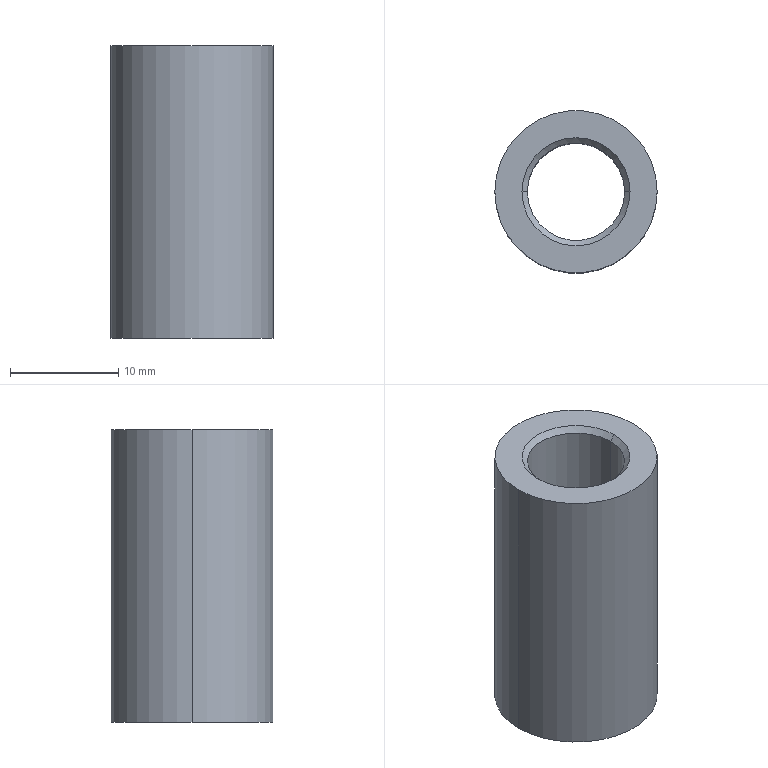Part | STEP file | Ngam kep 8 | 1 solid | 10 faces | box 15 x 15 x 27 mm | volume 3046 mm3 | cone 4 | cylinder 4 | plane 2 | commonest cylinder face diameters 9 x2 15 x2
STEP:
#1=CARTESIAN_POINT('',(0.,0.,0.));
#2=DIRECTION('',(0.,0.,1.));
#3=DIRECTION('',(1.,0.,0.));
#4=AXIS2_PLACEMENT_3D('',#1,#2,#3);
#5=CARTESIAN_POINT('',(4.5,0.,26.5));
#6=VERTEX_POINT('',#5);
#7=CARTESIAN_POINT('',(5.,0.,27.));
#8=VERTEX_POINT('',#7);
#9=CARTESIAN_POINT('',(4.5,0.,26.5));
#10=DIRECTION('',(0.7071,0.,0.7071));
#11=VECTOR('',#10,1.);
#12=LINE('',#9,#11);
#13=CARTESIAN_POINT('',(0.,0.,26.5));
#14=DIRECTION('',(0.,0.,1.));
#15=DIRECTION('',(1.,0.,0.));
#16=AXIS2_PLACEMENT_3D('',#13,#14,#15);
#17=CONICAL_SURFACE('',#16,4.5,0.7854);
#18=CARTESIAN_POINT('',(6.283,0.));
#19=DIRECTION('',(0.,1.));
#20=VECTOR('',#19,1.);
#21=LINE('',#18,#20);
#22=(GEOMETRIC_REPRESENTATION_CONTEXT(2)PARAMETRIC_REPRESENTATION_CONTEXT()REPRESENTATION_CONTEXT('',''));
#23=DEFINITIONAL_REPRESENTATION('',(#21),#22);
#24=PCURVE('',#17,#23);
#25=CARTESIAN_POINT('',(0.,0.,26.5));
#26=DIRECTION('',(0.,0.,1.));
#27=DIRECTION('',(1.,0.,0.));
#28=AXIS2_PLACEMENT_3D('',#25,#26,#27);
#29=CONICAL_SURFACE('',#28,4.5,0.7854);
#30=CARTESIAN_POINT('',(0.,0.));
#31=DIRECTION('',(0.,1.));
#32=VECTOR('',#31,1.);
#33=LINE('',#30,#32);
#34=(GEOMETRIC_REPRESENTATION_CONTEXT(2)PARAMETRIC_REPRESENTATION_CONTEXT()REPRESENTATION_CONTEXT('',''));
#35=DEFINITIONAL_REPRESENTATION('',(#33),#34);
#36=PCURVE('',#29,#35);
#37=SURFACE_CURVE('',#12,(#24,#36),.PCURVE_S1.);
#38=EDGE_CURVE('',#6,#8,#37,.T.);
#39=ORIENTED_EDGE('',*,*,#38,.T.);
#40=CARTESIAN_POINT('',(-5.,0.,27.));
#41=VERTEX_POINT('',#40);
#42=CARTESIAN_POINT('',(0.,0.,27.));
#43=DIRECTION('',(0.,0.,-1.));
#44=DIRECTION('',(1.,0.,0.));
#45=AXIS2_PLACEMENT_3D('',#42,#43,#44);
#46=CIRCLE('',#45,5.);
#47=CARTESIAN_POINT('',(6.283,0.5));
#48=DIRECTION('',(-1.,0.));
#49=VECTOR('',#48,1.);
#50=LINE('',#47,#49);
#51=(GEOMETRIC_REPRESENTATION_CONTEXT(2)PARAMETRIC_REPRESENTATION_CONTEXT()REPRESENTATION_CONTEXT('',''));
#52=DEFINITIONAL_REPRESENTATION('',(#50),#51);
#53=PCURVE('',#17,#52);
#54=CARTESIAN_POINT('',(0.,0.,27.));
#55=DIRECTION('',(0.,0.,1.));
#56=DIRECTION('',(1.,0.,0.));
#57=AXIS2_PLACEMENT_3D('',#54,#55,#56);
#58=PLANE('',#57);
#59=CARTESIAN_POINT('',(5.,0.));
#60=CARTESIAN_POINT('',(5.,-8.66));
#61=CARTESIAN_POINT('',(-2.5,-4.33));
#62=CARTESIAN_POINT('',(-10.,0.));
#63=CARTESIAN_POINT('',(-2.5,4.33));
#64=CARTESIAN_POINT('',(5.,8.66));
#65=CARTESIAN_POINT('',(5.,0.));
#66=(BOUNDED_CURVE()B_SPLINE_CURVE(2,(#59,#60,#61,#62,#63,#64,#65),.UNSPECIFIED.,.T.,.F.)B_SPLINE_CURVE_WITH_KNOTS((1,2,2,2,2,1),(-2.094,0.,2.094,4.189,6.283,8.378),.UNSPECIFIED.)CURVE()GEOMETRIC_REPRESENTATION_ITEM()RATIONAL_B_SPLINE_CURVE((1.,0.5,1.,0.5,1.,0.5,1.))REPRESENTATION_ITEM(''));
#67=(GEOMETRIC_REPRESENTATION_CONTEXT(2)PARAMETRIC_REPRESENTATION_CONTEXT()REPRESENTATION_CONTEXT('',''));
#68=DEFINITIONAL_REPRESENTATION('',(#66),#67);
#69=PCURVE('',#58,#68);
#70=SURFACE_CURVE('',#46,(#53,#69),.PCURVE_S1.);
#71=EDGE_CURVE('',#8,#41,#70,.T.);
#72=ORIENTED_EDGE('',*,*,#71,.T.);
#73=CARTESIAN_POINT('',(-4.5,0.,26.5));
#74=VERTEX_POINT('',#73);
#75=CARTESIAN_POINT('',(-4.5,0.,26.5));
#76=DIRECTION('',(-0.7071,0.,0.7071));
#77=VECTOR('',#76,1.);
#78=LINE('',#75,#77);
#79=CARTESIAN_POINT('',(3.142,0.));
#80=DIRECTION('',(0.,1.));
#81=VECTOR('',#80,1.);
#82=LINE('',#79,#81);
#83=(GEOMETRIC_REPRESENTATION_CONTEXT(2)PARAMETRIC_REPRESENTATION_CONTEXT()REPRESENTATION_CONTEXT('',''));
#84=DEFINITIONAL_REPRESENTATION('',(#82),#83);
#85=PCURVE('',#17,#84);
#86=CARTESIAN_POINT('',(3.142,0.));
#87=DIRECTION('',(0.,1.));
#88=VECTOR('',#87,1.);
#89=LINE('',#86,#88);
#90=(GEOMETRIC_REPRESENTATION_CONTEXT(2)PARAMETRIC_REPRESENTATION_CONTEXT()REPRESENTATION_CONTEXT('',''));
#91=DEFINITIONAL_REPRESENTATION('',(#89),#90);
#92=PCURVE('',#29,#91);
#93=SURFACE_CURVE('',#78,(#85,#92),.PCURVE_S1.);
#94=EDGE_CURVE('',#74,#41,#93,.T.);
#95=ORIENTED_EDGE('',*,*,#94,.F.);
#96=CARTESIAN_POINT('',(0.,0.,26.5));
#97=DIRECTION('',(0.,0.,1.));
#98=DIRECTION('',(1.,0.,0.));
#99=AXIS2_PLACEMENT_3D('',#96,#97,#98);
#100=CIRCLE('',#99,4.5);
#101=CARTESIAN_POINT('',(0.,0.));
#102=DIRECTION('',(1.,0.));
#103=VECTOR('',#102,1.);
#104=LINE('',#101,#103);
#105=(GEOMETRIC_REPRESENTATION_CONTEXT(2)PARAMETRIC_REPRESENTATION_CONTEXT()REPRESENTATION_CONTEXT('',''));
#106=DEFINITIONAL_REPRESENTATION('',(#104),#105);
#107=PCURVE('',#17,#106);
#108=CARTESIAN_POINT('',(0.,0.,27.));
#109=DIRECTION('',(0.,0.,-1.));
#110=DIRECTION('',(-1.,0.,0.));
#111=AXIS2_PLACEMENT_3D('',#108,#109,#110);
#112=CYLINDRICAL_SURFACE('',#111,4.5);
#113=CARTESIAN_POINT('',(9.425,0.5));
#114=DIRECTION('',(-1.,0.));
#115=VECTOR('',#114,1.);
#116=LINE('',#113,#115);
#117=(GEOMETRIC_REPRESENTATION_CONTEXT(2)PARAMETRIC_REPRESENTATION_CONTEXT()REPRESENTATION_CONTEXT('',''));
#118=DEFINITIONAL_REPRESENTATION('',(#116),#117);
#119=PCURVE('',#112,#118);
#120=SURFACE_CURVE('',#100,(#107,#119),.PCURVE_S1.);
#121=EDGE_CURVE('',#74,#6,#120,.T.);
#122=ORIENTED_EDGE('',*,*,#121,.T.);
#123=EDGE_LOOP('',(#39,#72,#95,#122));
#124=FACE_BOUND('',#123,.F.);
#125=ADVANCED_FACE('',(#124),#17,.F.);
#126=CARTESIAN_POINT('',(-4.5,0.,0.5));
#127=VERTEX_POINT('',#126);
#128=CARTESIAN_POINT('',(-5.,0.,0.));
#129=VERTEX_POINT('',#128);
#130=CARTESIAN_POINT('',(-5.,0.,0.));
#131=DIRECTION('',(-0.7071,0.,-0.7071));
#132=VECTOR('',#131,1.);
#133=LINE('',#130,#132);
#134=CARTESIAN_POINT('',(0.,0.,0.));
#135=DIRECTION('',(0.,0.,-1.));
#136=DIRECTION('',(-1.,0.,0.));
#137=AXIS2_PLACEMENT_3D('',#134,#135,#136);
#138=CONICAL_SURFACE('',#137,5.,0.7854);
#139=CARTESIAN_POINT('',(6.283,0.));
#140=DIRECTION('',(0.,1.));
#141=VECTOR('',#140,1.);
#142=LINE('',#139,#141);
#143=(GEOMETRIC_REPRESENTATION_CONTEXT(2)PARAMETRIC_REPRESENTATION_CONTEXT()REPRESENTATION_CONTEXT('',''));
#144=DEFINITIONAL_REPRESENTATION('',(#142),#143);
#145=PCURVE('',#138,#144);
#146=CARTESIAN_POINT('',(0.,0.,0.));
#147=DIRECTION('',(0.,0.,-1.));
#148=DIRECTION('',(-1.,0.,0.));
#149=AXIS2_PLACEMENT_3D('',#146,#147,#148);
#150=CONICAL_SURFACE('',#149,5.,0.7854);
#151=CARTESIAN_POINT('',(0.,0.));
#152=DIRECTION('',(0.,1.));
#153=VECTOR('',#152,1.);
#154=LINE('',#151,#153);
#155=(GEOMETRIC_REPRESENTATION_CONTEXT(2)PARAMETRIC_REPRESENTATION_CONTEXT()REPRESENTATION_CONTEXT('',''));
#156=DEFINITIONAL_REPRESENTATION('',(#154),#155);
#157=PCURVE('',#150,#156);
#158=SURFACE_CURVE('',#133,(#145,#157),.PCURVE_S1.);
#159=EDGE_CURVE('',#127,#129,#158,.T.);
#160=ORIENTED_EDGE('',*,*,#159,.T.);
#161=CARTESIAN_POINT('',(5.,0.,0.));
#162=VERTEX_POINT('',#161);
#163=CARTESIAN_POINT('',(0.,0.,0.));
#164=DIRECTION('',(0.,0.,1.));
#165=DIRECTION('',(1.,0.,0.));
#166=AXIS2_PLACEMENT_3D('',#163,#164,#165);
#167=CIRCLE('',#166,5.);
#168=CARTESIAN_POINT('',(9.425,0.));
#169=DIRECTION('',(-1.,0.));
#170=VECTOR('',#169,1.);
#171=LINE('',#168,#170);
#172=(GEOMETRIC_REPRESENTATION_CONTEXT(2)PARAMETRIC_REPRESENTATION_CONTEXT()REPRESENTATION_CONTEXT('',''));
#173=DEFINITIONAL_REPRESENTATION('',(#171),#172);
#174=PCURVE('',#138,#173);
#175=CARTESIAN_POINT('',(0.,0.,0.));
#176=DIRECTION('',(0.,0.,1.));
#177=DIRECTION('',(1.,0.,0.));
#178=AXIS2_PLACEMENT_3D('',#175,#176,#177);
#179=PLANE('',#178);
#180=CARTESIAN_POINT('',(0.,0.));
#181=DIRECTION('',(1.,0.));
#182=AXIS2_PLACEMENT_2D('',#180,#181);
#183=CIRCLE('',#182,5.);
#184=(GEOMETRIC_REPRESENTATION_CONTEXT(2)PARAMETRIC_REPRESENTATION_CONTEXT()REPRESENTATION_CONTEXT('',''));
#185=DEFINITIONAL_REPRESENTATION('',(#183),#184);
#186=PCURVE('',#179,#185);
#187=SURFACE_CURVE('',#167,(#174,#186),.PCURVE_S1.);
#188=EDGE_CURVE('',#129,#162,#187,.T.);
#189=ORIENTED_EDGE('',*,*,#188,.T.);
#190=CARTESIAN_POINT('',(4.5,0.,0.5));
#191=VERTEX_POINT('',#190);
#192=CARTESIAN_POINT('',(5.,0.,0.));
#193=DIRECTION('',(0.7071,0.,-0.7071));
#194=VECTOR('',#193,1.);
#195=LINE('',#192,#194);
#196=CARTESIAN_POINT('',(3.142,0.));
#197=DIRECTION('',(0.,1.));
#198=VECTOR('',#197,1.);
#199=LINE('',#196,#198);
#200=(GEOMETRIC_REPRESENTATION_CONTEXT(2)PARAMETRIC_REPRESENTATION_CONTEXT()REPRESENTATION_CONTEXT('',''));
#201=DEFINITIONAL_REPRESENTATION('',(#199),#200);
#202=PCURVE('',#138,#201);
#203=CARTESIAN_POINT('',(3.142,0.));
#204=DIRECTION('',(0.,1.));
#205=VECTOR('',#204,1.);
#206=LINE('',#203,#205);
#207=(GEOMETRIC_REPRESENTATION_CONTEXT(2)PARAMETRIC_REPRESENTATION_CONTEXT()REPRESENTATION_CONTEXT('',''));
#208=DEFINITIONAL_REPRESENTATION('',(#206),#207);
#209=PCURVE('',#150,#208);
#210=SURFACE_CURVE('',#195,(#202,#209),.PCURVE_S1.);
#211=EDGE_CURVE('',#191,#162,#210,.T.);
#212=ORIENTED_EDGE('',*,*,#211,.F.);
#213=CARTESIAN_POINT('',(0.,0.,0.5));
#214=DIRECTION('',(0.,0.,-1.));
#215=DIRECTION('',(1.,0.,0.));
#216=AXIS2_PLACEMENT_3D('',#213,#214,#215);
#217=CIRCLE('',#216,4.5);
#218=CARTESIAN_POINT('',(3.142,-0.5));
#219=DIRECTION('',(1.,0.));
#220=VECTOR('',#219,1.);
#221=LINE('',#218,#220);
#222=(GEOMETRIC_REPRESENTATION_CONTEXT(2)PARAMETRIC_REPRESENTATION_CONTEXT()REPRESENTATION_CONTEXT('',''));
#223=DEFINITIONAL_REPRESENTATION('',(#221),#222);
#224=PCURVE('',#138,#223);
#225=CARTESIAN_POINT('',(3.142,26.5));
#226=DIRECTION('',(1.,0.));
#227=VECTOR('',#226,1.);
#228=LINE('',#225,#227);
#229=(GEOMETRIC_REPRESENTATION_CONTEXT(2)PARAMETRIC_REPRESENTATION_CONTEXT()REPRESENTATION_CONTEXT('',''));
#230=DEFINITIONAL_REPRESENTATION('',(#228),#229);
#231=PCURVE('',#112,#230);
#232=SURFACE_CURVE('',#217,(#224,#231),.PCURVE_S1.);
#233=EDGE_CURVE('',#191,#127,#232,.T.);
#234=ORIENTED_EDGE('',*,*,#233,.T.);
#235=EDGE_LOOP('',(#160,#189,#212,#234));
#236=FACE_BOUND('',#235,.F.);
#237=ADVANCED_FACE('',(#236),#138,.F.);
#238=CARTESIAN_POINT('',(-4.5,0.,27.));
#239=DIRECTION('',(0.,0.,-1.));
#240=VECTOR('',#239,1.);
#241=LINE('',#238,#240);
#242=CARTESIAN_POINT('',(6.283,0.));
#243=DIRECTION('',(0.,1.));
#244=VECTOR('',#243,1.);
#245=LINE('',#242,#244);
#246=(GEOMETRIC_REPRESENTATION_CONTEXT(2)PARAMETRIC_REPRESENTATION_CONTEXT()REPRESENTATION_CONTEXT('',''));
#247=DEFINITIONAL_REPRESENTATION('',(#245),#246);
#248=PCURVE('',#112,#247);
#249=CARTESIAN_POINT('',(0.,0.,27.));
#250=DIRECTION('',(0.,0.,-1.));
#251=DIRECTION('',(-1.,0.,0.));
#252=AXIS2_PLACEMENT_3D('',#249,#250,#251);
#253=CYLINDRICAL_SURFACE('',#252,4.5);
#254=CARTESIAN_POINT('',(0.,0.));
#255=DIRECTION('',(0.,1.));
#256=VECTOR('',#255,1.);
#257=LINE('',#254,#256);
#258=(GEOMETRIC_REPRESENTATION_CONTEXT(2)PARAMETRIC_REPRESENTATION_CONTEXT()REPRESENTATION_CONTEXT('',''));
#259=DEFINITIONAL_REPRESENTATION('',(#257),#258);
#260=PCURVE('',#253,#259);
#261=SURFACE_CURVE('',#241,(#248,#260),.PCURVE_S1.);
#262=EDGE_CURVE('',#74,#127,#261,.T.);
#263=ORIENTED_EDGE('',*,*,#262,.T.);
#264=ORIENTED_EDGE('',*,*,#233,.F.);
#265=CARTESIAN_POINT('',(4.5,0.,27.));
#266=DIRECTION('',(0.,0.,-1.));
#267=VECTOR('',#266,1.);
#268=LINE('',#265,#267);
#269=CARTESIAN_POINT('',(3.142,0.));
#270=DIRECTION('',(0.,1.));
#271=VECTOR('',#270,1.);
#272=LINE('',#269,#271);
#273=(GEOMETRIC_REPRESENTATION_CONTEXT(2)PARAMETRIC_REPRESENTATION_CONTEXT()REPRESENTATION_CONTEXT('',''));
#274=DEFINITIONAL_REPRESENTATION('',(#272),#273);
#275=PCURVE('',#112,#274);
#276=CARTESIAN_POINT('',(3.142,0.));
#277=DIRECTION('',(0.,1.));
#278=VECTOR('',#277,1.);
#279=LINE('',#276,#278);
#280=(GEOMETRIC_REPRESENTATION_CONTEXT(2)PARAMETRIC_REPRESENTATION_CONTEXT()REPRESENTATION_CONTEXT('',''));
#281=DEFINITIONAL_REPRESENTATION('',(#279),#280);
#282=PCURVE('',#253,#281);
#283=SURFACE_CURVE('',#268,(#275,#282),.PCURVE_S1.);
#284=EDGE_CURVE('',#6,#191,#283,.T.);
#285=ORIENTED_EDGE('',*,*,#284,.F.);
#286=ORIENTED_EDGE('',*,*,#121,.F.);
#287=EDGE_LOOP('',(#263,#264,#285,#286));
#288=FACE_BOUND('',#287,.F.);
#289=ADVANCED_FACE('',(#288),#112,.F.);
#290=CARTESIAN_POINT('',(7.5,0.,27.));
#291=VERTEX_POINT('',#290);
#292=CARTESIAN_POINT('',(-7.5,0.,27.));
#293=VERTEX_POINT('',#292);
#294=CARTESIAN_POINT('',(0.,0.,27.));
#295=DIRECTION('',(0.,0.,1.));
#296=DIRECTION('',(1.,0.,0.));
#297=AXIS2_PLACEMENT_3D('',#294,#295,#296);
#298=CIRCLE('',#297,7.5);
#299=CARTESIAN_POINT('',(0.,0.,27.));
#300=DIRECTION('',(0.,0.,-1.));
#301=DIRECTION('',(-1.,0.,0.));
#302=AXIS2_PLACEMENT_3D('',#299,#300,#301);
#303=CYLINDRICAL_SURFACE('',#302,7.5);
#304=CARTESIAN_POINT('',(3.142,0.));
#305=DIRECTION('',(-1.,0.));
#306=VECTOR('',#305,1.);
#307=LINE('',#304,#306);
#308=(GEOMETRIC_REPRESENTATION_CONTEXT(2)PARAMETRIC_REPRESENTATION_CONTEXT()REPRESENTATION_CONTEXT('',''));
#309=DEFINITIONAL_REPRESENTATION('',(#307),#308);
#310=PCURVE('',#303,#309);
#311=CARTESIAN_POINT('',(0.,0.));
#312=DIRECTION('',(1.,0.));
#313=AXIS2_PLACEMENT_2D('',#311,#312);
#314=CIRCLE('',#313,7.5);
#315=(GEOMETRIC_REPRESENTATION_CONTEXT(2)PARAMETRIC_REPRESENTATION_CONTEXT()REPRESENTATION_CONTEXT('',''));
#316=DEFINITIONAL_REPRESENTATION('',(#314),#315);
#317=PCURVE('',#58,#316);
#318=SURFACE_CURVE('',#298,(#310,#317),.PCURVE_S1.);
#319=EDGE_CURVE('',#291,#293,#318,.T.);
#320=ORIENTED_EDGE('',*,*,#319,.F.);
#321=CARTESIAN_POINT('',(7.5,0.,0.));
#322=VERTEX_POINT('',#321);
#323=CARTESIAN_POINT('',(7.5,0.,27.));
#324=DIRECTION('',(0.,0.,-1.));
#325=VECTOR('',#324,1.);
#326=LINE('',#323,#325);
#327=CARTESIAN_POINT('',(3.142,0.));
#328=DIRECTION('',(0.,1.));
#329=VECTOR('',#328,1.);
#330=LINE('',#327,#329);
#331=(GEOMETRIC_REPRESENTATION_CONTEXT(2)PARAMETRIC_REPRESENTATION_CONTEXT()REPRESENTATION_CONTEXT('',''));
#332=DEFINITIONAL_REPRESENTATION('',(#330),#331);
#333=PCURVE('',#303,#332);
#334=CARTESIAN_POINT('',(0.,0.,27.));
#335=DIRECTION('',(0.,0.,-1.));
#336=DIRECTION('',(-1.,0.,0.));
#337=AXIS2_PLACEMENT_3D('',#334,#335,#336);
#338=CYLINDRICAL_SURFACE('',#337,7.5);
#339=CARTESIAN_POINT('',(3.142,0.));
#340=DIRECTION('',(0.,1.));
#341=VECTOR('',#340,1.);
#342=LINE('',#339,#341);
#343=(GEOMETRIC_REPRESENTATION_CONTEXT(2)PARAMETRIC_REPRESENTATION_CONTEXT()REPRESENTATION_CONTEXT('',''));
#344=DEFINITIONAL_REPRESENTATION('',(#342),#343);
#345=PCURVE('',#338,#344);
#346=SURFACE_CURVE('',#326,(#333,#345),.PCURVE_S1.);
#347=EDGE_CURVE('',#291,#322,#346,.T.);
#348=ORIENTED_EDGE('',*,*,#347,.T.);
#349=CARTESIAN_POINT('',(-7.5,0.,0.));
#350=VERTEX_POINT('',#349);
#351=CARTESIAN_POINT('',(0.,0.,0.));
#352=DIRECTION('',(0.,0.,1.));
#353=DIRECTION('',(1.,0.,0.));
#354=AXIS2_PLACEMENT_3D('',#351,#352,#353);
#355=CIRCLE('',#354,7.5);
#356=CARTESIAN_POINT('',(3.142,27.));
#357=DIRECTION('',(-1.,0.));
#358=VECTOR('',#357,1.);
#359=LINE('',#356,#358);
#360=(GEOMETRIC_REPRESENTATION_CONTEXT(2)PARAMETRIC_REPRESENTATION_CONTEXT()REPRESENTATION_CONTEXT('',''));
#361=DEFINITIONAL_REPRESENTATION('',(#359),#360);
#362=PCURVE('',#303,#361);
#363=CARTESIAN_POINT('',(0.,0.));
#364=DIRECTION('',(1.,0.));
#365=AXIS2_PLACEMENT_2D('',#363,#364);
#366=CIRCLE('',#365,7.5);
#367=(GEOMETRIC_REPRESENTATION_CONTEXT(2)PARAMETRIC_REPRESENTATION_CONTEXT()REPRESENTATION_CONTEXT('',''));
#368=DEFINITIONAL_REPRESENTATION('',(#366),#367);
#369=PCURVE('',#179,#368);
#370=SURFACE_CURVE('',#355,(#362,#369),.PCURVE_S1.);
#371=EDGE_CURVE('',#322,#350,#370,.T.);
#372=ORIENTED_EDGE('',*,*,#371,.T.);
#373=CARTESIAN_POINT('',(-7.5,0.,27.));
#374=DIRECTION('',(0.,0.,-1.));
#375=VECTOR('',#374,1.);
#376=LINE('',#373,#375);
#377=CARTESIAN_POINT('',(0.,0.));
#378=DIRECTION('',(0.,1.));
#379=VECTOR('',#378,1.);
#380=LINE('',#377,#379);
#381=(GEOMETRIC_REPRESENTATION_CONTEXT(2)PARAMETRIC_REPRESENTATION_CONTEXT()REPRESENTATION_CONTEXT('',''));
#382=DEFINITIONAL_REPRESENTATION('',(#380),#381);
#383=PCURVE('',#303,#382);
#384=CARTESIAN_POINT('',(6.283,0.));
#385=DIRECTION('',(0.,1.));
#386=VECTOR('',#385,1.);
#387=LINE('',#384,#386);
#388=(GEOMETRIC_REPRESENTATION_CONTEXT(2)PARAMETRIC_REPRESENTATION_CONTEXT()REPRESENTATION_CONTEXT('',''));
#389=DEFINITIONAL_REPRESENTATION('',(#387),#388);
#390=PCURVE('',#338,#389);
#391=SURFACE_CURVE('',#376,(#383,#390),.PCURVE_S1.);
#392=EDGE_CURVE('',#293,#350,#391,.T.);
#393=ORIENTED_EDGE('',*,*,#392,.F.);
#394=EDGE_LOOP('',(#320,#348,#372,#393));
#395=FACE_BOUND('',#394,.T.);
#396=ADVANCED_FACE('',(#395),#303,.T.);
#397=ORIENTED_EDGE('',*,*,#71,.T.);
#398=CARTESIAN_POINT('',(0.,0.,27.));
#399=DIRECTION('',(0.,0.,-1.));
#400=DIRECTION('',(1.,0.,0.));
#401=AXIS2_PLACEMENT_3D('',#398,#399,#400);
#402=CIRCLE('',#401,5.);
#403=CARTESIAN_POINT('',(5.,0.));
#404=CARTESIAN_POINT('',(5.,-8.66));
#405=CARTESIAN_POINT('',(-2.5,-4.33));
#406=CARTESIAN_POINT('',(-10.,0.));
#407=CARTESIAN_POINT('',(-2.5,4.33));
#408=CARTESIAN_POINT('',(5.,8.66));
#409=CARTESIAN_POINT('',(5.,0.));
#410=(BOUNDED_CURVE()B_SPLINE_CURVE(2,(#403,#404,#405,#406,#407,#408,#409),.UNSPECIFIED.,.T.,.F.)B_SPLINE_CURVE_WITH_KNOTS((1,2,2,2,2,1),(-2.094,0.,2.094,4.189,6.283,8.378),.UNSPECIFIED.)CURVE()GEOMETRIC_REPRESENTATION_ITEM()RATIONAL_B_SPLINE_CURVE((1.,0.5,1.,0.5,1.,0.5,1.))REPRESENTATION_ITEM(''));
#411=(GEOMETRIC_REPRESENTATION_CONTEXT(2)PARAMETRIC_REPRESENTATION_CONTEXT()REPRESENTATION_CONTEXT('',''));
#412=DEFINITIONAL_REPRESENTATION('',(#410),#411);
#413=PCURVE('',#58,#412);
#414=CARTESIAN_POINT('',(6.283,0.5));
#415=DIRECTION('',(-1.,0.));
#416=VECTOR('',#415,1.);
#417=LINE('',#414,#416);
#418=(GEOMETRIC_REPRESENTATION_CONTEXT(2)PARAMETRIC_REPRESENTATION_CONTEXT()REPRESENTATION_CONTEXT('',''));
#419=DEFINITIONAL_REPRESENTATION('',(#417),#418);
#420=PCURVE('',#29,#419);
#421=SURFACE_CURVE('',#402,(#413,#420),.PCURVE_S1.);
#422=EDGE_CURVE('',#41,#8,#421,.T.);
#423=ORIENTED_EDGE('',*,*,#422,.T.);
#424=EDGE_LOOP('',(#397,#423));
#425=FACE_BOUND('',#424,.T.);
#426=CARTESIAN_POINT('',(0.,0.,27.));
#427=DIRECTION('',(0.,0.,1.));
#428=DIRECTION('',(1.,0.,0.));
#429=AXIS2_PLACEMENT_3D('',#426,#427,#428);
#430=CIRCLE('',#429,7.5);
#431=CARTESIAN_POINT('',(0.,0.));
#432=DIRECTION('',(1.,0.));
#433=AXIS2_PLACEMENT_2D('',#431,#432);
#434=CIRCLE('',#433,7.5);
#435=(GEOMETRIC_REPRESENTATION_CONTEXT(2)PARAMETRIC_REPRESENTATION_CONTEXT()REPRESENTATION_CONTEXT('',''));
#436=DEFINITIONAL_REPRESENTATION('',(#434),#435);
#437=PCURVE('',#58,#436);
#438=CARTESIAN_POINT('',(9.425,0.));
#439=DIRECTION('',(-1.,0.));
#440=VECTOR('',#439,1.);
#441=LINE('',#438,#440);
#442=(GEOMETRIC_REPRESENTATION_CONTEXT(2)PARAMETRIC_REPRESENTATION_CONTEXT()REPRESENTATION_CONTEXT('',''));
#443=DEFINITIONAL_REPRESENTATION('',(#441),#442);
#444=PCURVE('',#338,#443);
#445=SURFACE_CURVE('',#430,(#437,#444),.PCURVE_S1.);
#446=EDGE_CURVE('',#293,#291,#445,.T.);
#447=ORIENTED_EDGE('',*,*,#446,.T.);
#448=ORIENTED_EDGE('',*,*,#319,.T.);
#449=EDGE_LOOP('',(#447,#448));
#450=FACE_BOUND('',#449,.T.);
#451=ADVANCED_FACE('',(#425,#450),#58,.T.);
#452=ORIENTED_EDGE('',*,*,#188,.T.);
#453=CARTESIAN_POINT('',(0.,0.,0.));
#454=DIRECTION('',(0.,0.,1.));
#455=DIRECTION('',(1.,0.,0.));
#456=AXIS2_PLACEMENT_3D('',#453,#454,#455);
#457=CIRCLE('',#456,5.);
#458=CARTESIAN_POINT('',(0.,0.));
#459=DIRECTION('',(1.,0.));
#460=AXIS2_PLACEMENT_2D('',#458,#459);
#461=CIRCLE('',#460,5.);
#462=(GEOMETRIC_REPRESENTATION_CONTEXT(2)PARAMETRIC_REPRESENTATION_CONTEXT()REPRESENTATION_CONTEXT('',''));
#463=DEFINITIONAL_REPRESENTATION('',(#461),#462);
#464=PCURVE('',#179,#463);
#465=CARTESIAN_POINT('',(3.142,0.));
#466=DIRECTION('',(-1.,0.));
#467=VECTOR('',#466,1.);
#468=LINE('',#465,#467);
#469=(GEOMETRIC_REPRESENTATION_CONTEXT(2)PARAMETRIC_REPRESENTATION_CONTEXT()REPRESENTATION_CONTEXT('',''));
#470=DEFINITIONAL_REPRESENTATION('',(#468),#469);
#471=PCURVE('',#150,#470);
#472=SURFACE_CURVE('',#457,(#464,#471),.PCURVE_S1.);
#473=EDGE_CURVE('',#162,#129,#472,.T.);
#474=ORIENTED_EDGE('',*,*,#473,.T.);
#475=EDGE_LOOP('',(#452,#474));
#476=FACE_BOUND('',#475,.T.);
#477=CARTESIAN_POINT('',(0.,0.,0.));
#478=DIRECTION('',(0.,0.,1.));
#479=DIRECTION('',(1.,0.,0.));
#480=AXIS2_PLACEMENT_3D('',#477,#478,#479);
#481=CIRCLE('',#480,7.5);
#482=CARTESIAN_POINT('',(0.,0.));
#483=DIRECTION('',(1.,0.));
#484=AXIS2_PLACEMENT_2D('',#482,#483);
#485=CIRCLE('',#484,7.5);
#486=(GEOMETRIC_REPRESENTATION_CONTEXT(2)PARAMETRIC_REPRESENTATION_CONTEXT()REPRESENTATION_CONTEXT('',''));
#487=DEFINITIONAL_REPRESENTATION('',(#485),#486);
#488=PCURVE('',#179,#487);
#489=CARTESIAN_POINT('',(9.425,27.));
#490=DIRECTION('',(-1.,0.));
#491=VECTOR('',#490,1.);
#492=LINE('',#489,#491);
#493=(GEOMETRIC_REPRESENTATION_CONTEXT(2)PARAMETRIC_REPRESENTATION_CONTEXT()REPRESENTATION_CONTEXT('',''));
#494=DEFINITIONAL_REPRESENTATION('',(#492),#493);
#495=PCURVE('',#338,#494);
#496=SURFACE_CURVE('',#481,(#488,#495),.PCURVE_S1.);
#497=EDGE_CURVE('',#350,#322,#496,.T.);
#498=ORIENTED_EDGE('',*,*,#497,.F.);
#499=ORIENTED_EDGE('',*,*,#371,.F.);
#500=EDGE_LOOP('',(#498,#499));
#501=FACE_BOUND('',#500,.T.);
#502=ADVANCED_FACE('',(#476,#501),#179,.F.);
#503=ORIENTED_EDGE('',*,*,#347,.F.);
#504=ORIENTED_EDGE('',*,*,#446,.F.);
#505=ORIENTED_EDGE('',*,*,#392,.T.);
#506=ORIENTED_EDGE('',*,*,#497,.T.);
#507=EDGE_LOOP('',(#503,#504,#505,#506));
#508=FACE_BOUND('',#507,.T.);
#509=ADVANCED_FACE('',(#508),#338,.T.);
#510=CARTESIAN_POINT('',(0.,0.,0.5));
#511=DIRECTION('',(0.,0.,-1.));
#512=DIRECTION('',(1.,0.,0.));
#513=AXIS2_PLACEMENT_3D('',#510,#511,#512);
#514=CIRCLE('',#513,4.5);
#515=CARTESIAN_POINT('',(-3.142,26.5));
#516=DIRECTION('',(1.,0.));
#517=VECTOR('',#516,1.);
#518=LINE('',#515,#517);
#519=(GEOMETRIC_REPRESENTATION_CONTEXT(2)PARAMETRIC_REPRESENTATION_CONTEXT()REPRESENTATION_CONTEXT('',''));
#520=DEFINITIONAL_REPRESENTATION('',(#518),#519);
#521=PCURVE('',#253,#520);
#522=CARTESIAN_POINT('',(-3.142,-0.5));
#523=DIRECTION('',(1.,0.));
#524=VECTOR('',#523,1.);
#525=LINE('',#522,#524);
#526=(GEOMETRIC_REPRESENTATION_CONTEXT(2)PARAMETRIC_REPRESENTATION_CONTEXT()REPRESENTATION_CONTEXT('',''));
#527=DEFINITIONAL_REPRESENTATION('',(#525),#526);
#528=PCURVE('',#150,#527);
#529=SURFACE_CURVE('',#514,(#521,#528),.PCURVE_S1.);
#530=EDGE_CURVE('',#127,#191,#529,.T.);
#531=ORIENTED_EDGE('',*,*,#530,.F.);
#532=ORIENTED_EDGE('',*,*,#262,.F.);
#533=CARTESIAN_POINT('',(0.,0.,26.5));
#534=DIRECTION('',(0.,0.,1.));
#535=DIRECTION('',(1.,0.,0.));
#536=AXIS2_PLACEMENT_3D('',#533,#534,#535);
#537=CIRCLE('',#536,4.5);
#538=CARTESIAN_POINT('',(3.142,0.5));
#539=DIRECTION('',(-1.,0.));
#540=VECTOR('',#539,1.);
#541=LINE('',#538,#540);
#542=(GEOMETRIC_REPRESENTATION_CONTEXT(2)PARAMETRIC_REPRESENTATION_CONTEXT()REPRESENTATION_CONTEXT('',''));
#543=DEFINITIONAL_REPRESENTATION('',(#541),#542);
#544=PCURVE('',#253,#543);
#545=CARTESIAN_POINT('',(0.,0.));
#546=DIRECTION('',(1.,0.));
#547=VECTOR('',#546,1.);
#548=LINE('',#545,#547);
#549=(GEOMETRIC_REPRESENTATION_CONTEXT(2)PARAMETRIC_REPRESENTATION_CONTEXT()REPRESENTATION_CONTEXT('',''));
#550=DEFINITIONAL_REPRESENTATION('',(#548),#549);
#551=PCURVE('',#29,#550);
#552=SURFACE_CURVE('',#537,(#544,#551),.PCURVE_S1.);
#553=EDGE_CURVE('',#6,#74,#552,.T.);
#554=ORIENTED_EDGE('',*,*,#553,.F.);
#555=ORIENTED_EDGE('',*,*,#284,.T.);
#556=EDGE_LOOP('',(#531,#532,#554,#555));
#557=FACE_BOUND('',#556,.F.);
#558=ADVANCED_FACE('',(#557),#253,.F.);
#559=ORIENTED_EDGE('',*,*,#473,.T.);
#560=ORIENTED_EDGE('',*,*,#159,.F.);
#561=ORIENTED_EDGE('',*,*,#530,.T.);
#562=ORIENTED_EDGE('',*,*,#211,.T.);
#563=EDGE_LOOP('',(#559,#560,#561,#562));
#564=FACE_BOUND('',#563,.F.);
#565=ADVANCED_FACE('',(#564),#150,.F.);
#566=ORIENTED_EDGE('',*,*,#422,.T.);
#567=ORIENTED_EDGE('',*,*,#38,.F.);
#568=ORIENTED_EDGE('',*,*,#553,.T.);
#569=ORIENTED_EDGE('',*,*,#94,.T.);
#570=EDGE_LOOP('',(#566,#567,#568,#569));
#571=FACE_BOUND('',#570,.F.);
#572=ADVANCED_FACE('',(#571),#29,.F.);
#573=CLOSED_SHELL('',(#125,#237,#289,#396,#451,#502,#509,#558,#565,#572));
#574=MANIFOLD_SOLID_BREP('',#573);
#575=(LENGTH_UNIT()NAMED_UNIT(*)SI_UNIT(.MILLI.,.METRE.));
#576=UNCERTAINTY_MEASURE_WITH_UNIT(LENGTH_MEASURE(0.0000001),#575,'','');
#577=(NAMED_UNIT(*)PLANE_ANGLE_UNIT()SI_UNIT($,.RADIAN.));
#578=(NAMED_UNIT(*)SI_UNIT($,.STERADIAN.)SOLID_ANGLE_UNIT());
#579=(GEOMETRIC_REPRESENTATION_CONTEXT(3)GLOBAL_UNCERTAINTY_ASSIGNED_CONTEXT((#576))GLOBAL_UNIT_ASSIGNED_CONTEXT((#575,#577,#578))REPRESENTATION_CONTEXT('',''));
#580=ADVANCED_BREP_SHAPE_REPRESENTATION('',(#4,#574),#579);